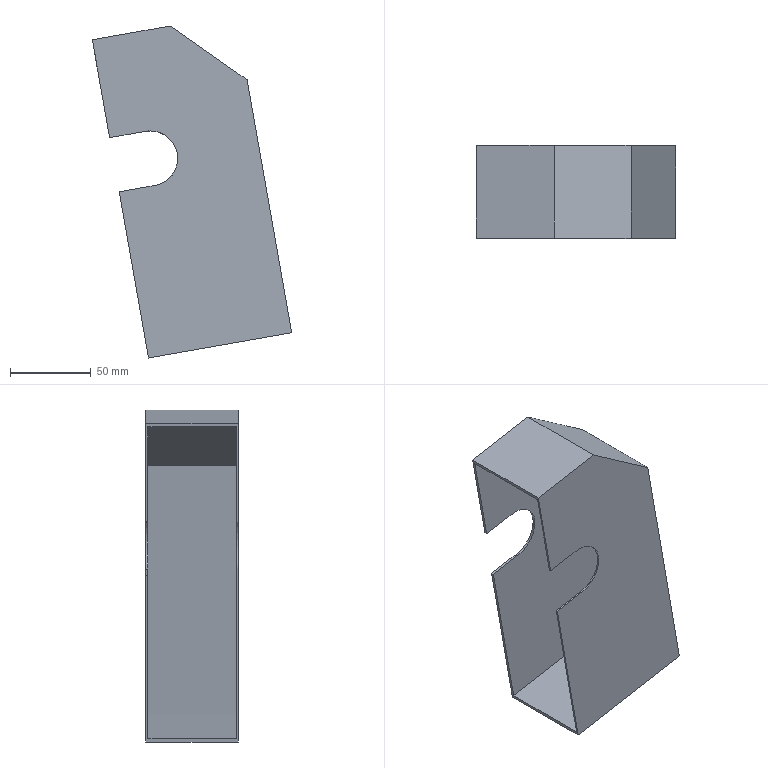Part | SolidWorks | features ICE 3, BaseBody 1, Cut 1 | 1 solid | 21 faces | box 123.362 x 57.5 x 205.47 mm | volume 78596 mm3 | plane 18 | cylinder 3 | commonest cylinder face diameters 34.017 x3
STEP:
#1=CARTESIAN_POINT('',(1.171,250.,328.559));
#2=VERTEX_POINT('',#1);
#3=CARTESIAN_POINT('',(4.125,250.,294.8));
#4=VERTEX_POINT('',#3);
#5=CARTESIAN_POINT('',(1.171,250.,311.55));
#6=DIRECTION('',(0.,1.,0.));
#7=DIRECTION('',(0.,0.,-1.));
#8=AXIS2_PLACEMENT_3D('',#5,#6,#7);
#9=CIRCLE('',#8,17.008);
#10=EDGE_CURVE('',#2,#4,#9,.T.);
#11=ORIENTED_EDGE('',*,*,#10,.F.);
#12=CARTESIAN_POINT('',(1.171,251.,328.559));
#13=VERTEX_POINT('',#12);
#14=CARTESIAN_POINT('',(1.171,191.5,328.559));
#15=DIRECTION('',(0.,1.,0.));
#16=VECTOR('',#15,1000.);
#17=LINE('',#14,#16);
#18=EDGE_CURVE('',#2,#13,#17,.T.);
#19=ORIENTED_EDGE('',*,*,#18,.T.);
#20=CARTESIAN_POINT('',(4.125,251.,294.8));
#21=VERTEX_POINT('',#20);
#22=CARTESIAN_POINT('',(1.171,251.,311.55));
#23=DIRECTION('',(0.,1.,0.));
#24=DIRECTION('',(0.,0.,-1.));
#25=AXIS2_PLACEMENT_3D('',#22,#23,#24);
#26=CIRCLE('',#25,17.008);
#27=EDGE_CURVE('',#13,#21,#26,.T.);
#28=ORIENTED_EDGE('',*,*,#27,.T.);
#29=CARTESIAN_POINT('',(4.125,191.5,294.8));
#30=DIRECTION('',(0.,1.,0.));
#31=VECTOR('',#30,1000.);
#32=LINE('',#29,#31);
#33=EDGE_CURVE('',#4,#21,#32,.T.);
#34=ORIENTED_EDGE('',*,*,#33,.F.);
#35=EDGE_LOOP('',(#11,#19,#28,#34));
#36=FACE_OUTER_BOUND('',#35,.T.);
#37=CARTESIAN_POINT('',(1.171,191.5,311.55));
#38=DIRECTION('',(0.,1.,0.));
#39=DIRECTION('',(0.,0.,1.));
#40=AXIS2_PLACEMENT_3D('',#37,#38,#39);
#41=CYLINDRICAL_SURFACE('',#40,17.008);
#42=ADVANCED_FACE('',(#36),#41,.F.);
#43=CARTESIAN_POINT('',(-18.14,251.,290.874));
#44=VERTEX_POINT('',#43);
#45=CARTESIAN_POINT('',(-18.14,250.,290.874));
#46=VERTEX_POINT('',#45);
#47=CARTESIAN_POINT('',(-18.14,0.,290.874));
#48=DIRECTION('',(0.,-1.,0.));
#49=VECTOR('',#48,1000.);
#50=LINE('',#47,#49);
#51=EDGE_CURVE('',#44,#46,#50,.T.);
#52=ORIENTED_EDGE('',*,*,#51,.F.);
#53=CARTESIAN_POINT('',(-0.3473,251.,189.97));
#54=VERTEX_POINT('',#53);
#55=CARTESIAN_POINT('',(-34.73,251.,384.962));
#56=DIRECTION('',(0.1736,0.,-0.9848));
#57=VECTOR('',#56,1000.);
#58=LINE('',#55,#57);
#59=EDGE_CURVE('',#44,#54,#58,.T.);
#60=ORIENTED_EDGE('',*,*,#59,.T.);
#61=CARTESIAN_POINT('',(-0.3473,306.,189.97));
#62=VERTEX_POINT('',#61);
#63=CARTESIAN_POINT('',(-0.3473,208.,189.97));
#64=DIRECTION('',(0.,1.,0.));
#65=VECTOR('',#64,1000.);
#66=LINE('',#63,#65);
#67=EDGE_CURVE('',#54,#62,#66,.T.);
#68=ORIENTED_EDGE('',*,*,#67,.T.);
#69=CARTESIAN_POINT('',(-18.14,306.,290.874));
#70=VERTEX_POINT('',#69);
#71=CARTESIAN_POINT('',(0.,306.,188.));
#72=DIRECTION('',(-0.1736,0.,0.9848));
#73=VECTOR('',#72,1000.);
#74=LINE('',#71,#73);
#75=EDGE_CURVE('',#62,#70,#74,.T.);
#76=ORIENTED_EDGE('',*,*,#75,.T.);
#77=CARTESIAN_POINT('',(-18.14,307.5,290.874));
#78=VERTEX_POINT('',#77);
#79=CARTESIAN_POINT('',(-18.14,0.,290.874));
#80=DIRECTION('',(0.,1.,0.));
#81=VECTOR('',#80,1000.);
#82=LINE('',#79,#81);
#83=EDGE_CURVE('',#70,#78,#82,.T.);
#84=ORIENTED_EDGE('',*,*,#83,.T.);
#85=CARTESIAN_POINT('',(0.,307.5,188.));
#86=VERTEX_POINT('',#85);
#87=CARTESIAN_POINT('',(0.,307.5,188.));
#88=DIRECTION('',(-0.1736,0.,0.9848));
#89=VECTOR('',#88,1000.);
#90=LINE('',#87,#89);
#91=EDGE_CURVE('',#86,#78,#90,.T.);
#92=ORIENTED_EDGE('',*,*,#91,.F.);
#93=CARTESIAN_POINT('',(0.,250.,188.));
#94=VERTEX_POINT('',#93);
#95=CARTESIAN_POINT('',(0.,208.,188.));
#96=DIRECTION('',(0.,1.,0.));
#97=VECTOR('',#96,1000.);
#98=LINE('',#95,#97);
#99=EDGE_CURVE('',#94,#86,#98,.T.);
#100=ORIENTED_EDGE('',*,*,#99,.F.);
#101=CARTESIAN_POINT('',(-34.73,250.,384.962));
#102=DIRECTION('',(0.1736,0.,-0.9848));
#103=VECTOR('',#102,1000.);
#104=LINE('',#101,#103);
#105=EDGE_CURVE('',#46,#94,#104,.T.);
#106=ORIENTED_EDGE('',*,*,#105,.F.);
#107=EDGE_LOOP('',(#52,#60,#68,#76,#84,#92,#100,#106));
#108=FACE_OUTER_BOUND('',#107,.T.);
#109=CARTESIAN_POINT('',(0.,0.,188.));
#110=DIRECTION('',(0.9848,0.,0.1736));
#111=DIRECTION('',(-0.1736,0.,0.9848));
#112=AXIS2_PLACEMENT_3D('',#109,#110,#111);
#113=PLANE('',#112);
#114=ADVANCED_FACE('',(#108),#113,.F.);
#115=CARTESIAN_POINT('',(-24.046,250.,324.374));
#116=VERTEX_POINT('',#115);
#117=CARTESIAN_POINT('',(-24.046,251.,324.374));
#118=VERTEX_POINT('',#117);
#119=CARTESIAN_POINT('',(-24.046,0.,324.374));
#120=DIRECTION('',(0.,1.,0.));
#121=VECTOR('',#120,1000.);
#122=LINE('',#119,#121);
#123=EDGE_CURVE('',#116,#118,#122,.T.);
#124=ORIENTED_EDGE('',*,*,#123,.F.);
#125=CARTESIAN_POINT('',(-34.73,250.,384.962));
#126=VERTEX_POINT('',#125);
#127=CARTESIAN_POINT('',(-34.73,250.,384.962));
#128=DIRECTION('',(0.1736,0.,-0.9848));
#129=VECTOR('',#128,1000.);
#130=LINE('',#127,#129);
#131=EDGE_CURVE('',#126,#116,#130,.T.);
#132=ORIENTED_EDGE('',*,*,#131,.F.);
#133=CARTESIAN_POINT('',(-34.73,307.5,384.962));
#134=VERTEX_POINT('',#133);
#135=CARTESIAN_POINT('',(-34.73,298.,384.962));
#136=DIRECTION('',(0.,-1.,0.));
#137=VECTOR('',#136,1000.);
#138=LINE('',#135,#137);
#139=EDGE_CURVE('',#134,#126,#138,.T.);
#140=ORIENTED_EDGE('',*,*,#139,.F.);
#141=CARTESIAN_POINT('',(-24.046,307.5,324.374));
#142=VERTEX_POINT('',#141);
#143=CARTESIAN_POINT('',(-24.046,307.5,324.374));
#144=DIRECTION('',(-0.1736,0.,0.9848));
#145=VECTOR('',#144,1000.);
#146=LINE('',#143,#145);
#147=EDGE_CURVE('',#142,#134,#146,.T.);
#148=ORIENTED_EDGE('',*,*,#147,.F.);
#149=CARTESIAN_POINT('',(-24.046,306.,324.374));
#150=VERTEX_POINT('',#149);
#151=CARTESIAN_POINT('',(-24.046,0.,324.374));
#152=DIRECTION('',(0.,-1.,0.));
#153=VECTOR('',#152,1000.);
#154=LINE('',#151,#153);
#155=EDGE_CURVE('',#142,#150,#154,.T.);
#156=ORIENTED_EDGE('',*,*,#155,.T.);
#157=CARTESIAN_POINT('',(-34.382,306.,382.992));
#158=VERTEX_POINT('',#157);
#159=CARTESIAN_POINT('',(0.,306.,188.));
#160=DIRECTION('',(-0.1736,0.,0.9848));
#161=VECTOR('',#160,1000.);
#162=LINE('',#159,#161);
#163=EDGE_CURVE('',#150,#158,#162,.T.);
#164=ORIENTED_EDGE('',*,*,#163,.T.);
#165=CARTESIAN_POINT('',(-34.382,251.,382.992));
#166=VERTEX_POINT('',#165);
#167=CARTESIAN_POINT('',(-34.382,298.,382.992));
#168=DIRECTION('',(0.,-1.,0.));
#169=VECTOR('',#168,1000.);
#170=LINE('',#167,#169);
#171=EDGE_CURVE('',#158,#166,#170,.T.);
#172=ORIENTED_EDGE('',*,*,#171,.T.);
#173=CARTESIAN_POINT('',(-34.73,251.,384.962));
#174=DIRECTION('',(0.1736,0.,-0.9848));
#175=VECTOR('',#174,1000.);
#176=LINE('',#173,#175);
#177=EDGE_CURVE('',#166,#118,#176,.T.);
#178=ORIENTED_EDGE('',*,*,#177,.T.);
#179=EDGE_LOOP('',(#124,#132,#140,#148,#156,#164,#172,#178));
#180=FACE_OUTER_BOUND('',#179,.T.);
#181=CARTESIAN_POINT('',(0.,0.,188.));
#182=DIRECTION('',(0.9848,0.,0.1736));
#183=DIRECTION('',(-0.1736,0.,0.9848));
#184=AXIS2_PLACEMENT_3D('',#181,#182,#183);
#185=PLANE('',#184);
#186=ADVANCED_FACE('',(#180),#185,.F.);
#187=CARTESIAN_POINT('',(-50.289,251.,285.205));
#188=DIRECTION('',(-0.9848,0.,-0.1736));
#189=VECTOR('',#188,1000.);
#190=LINE('',#187,#189);
#191=EDGE_CURVE('',#21,#44,#190,.T.);
#192=ORIENTED_EDGE('',*,*,#191,.F.);
#193=ORIENTED_EDGE('',*,*,#27,.F.);
#194=CARTESIAN_POINT('',(-1.782,251.,328.3));
#195=VERTEX_POINT('',#194);
#196=CARTESIAN_POINT('',(1.171,251.,311.55));
#197=DIRECTION('',(0.,1.,0.));
#198=DIRECTION('',(0.,0.,-1.));
#199=AXIS2_PLACEMENT_3D('',#196,#197,#198);
#200=CIRCLE('',#199,17.008);
#201=EDGE_CURVE('',#195,#13,#200,.T.);
#202=ORIENTED_EDGE('',*,*,#201,.F.);
#203=CARTESIAN_POINT('',(-56.196,251.,318.706));
#204=DIRECTION('',(0.9848,0.,0.1736));
#205=VECTOR('',#204,1000.);
#206=LINE('',#203,#205);
#207=EDGE_CURVE('',#118,#195,#206,.T.);
#208=ORIENTED_EDGE('',*,*,#207,.F.);
#209=ORIENTED_EDGE('',*,*,#177,.F.);
#210=CARTESIAN_POINT('',(13.057,251.,391.357));
#211=VERTEX_POINT('',#210);
#212=CARTESIAN_POINT('',(54.25,251.,398.62));
#213=DIRECTION('',(-0.9848,0.,-0.1736));
#214=VECTOR('',#213,1000.);
#215=LINE('',#212,#214);
#216=EDGE_CURVE('',#211,#166,#215,.T.);
#217=ORIENTED_EDGE('',*,*,#216,.F.);
#218=CARTESIAN_POINT('',(59.197,251.,359.05));
#219=VERTEX_POINT('',#218);
#220=CARTESIAN_POINT('',(59.875,251.,358.574));
#221=DIRECTION('',(0.8192,0.,-0.5736));
#222=VECTOR('',#221,1000.);
#223=LINE('',#220,#222);
#224=EDGE_CURVE('',#211,#219,#223,.T.);
#225=ORIENTED_EDGE('',*,*,#224,.T.);
#226=CARTESIAN_POINT('',(86.316,251.,205.251));
#227=VERTEX_POINT('',#226);
#228=CARTESIAN_POINT('',(86.663,251.,203.281));
#229=DIRECTION('',(0.1736,0.,-0.9848));
#230=VECTOR('',#229,1000.);
#231=LINE('',#228,#230);
#232=EDGE_CURVE('',#219,#227,#231,.T.);
#233=ORIENTED_EDGE('',*,*,#232,.T.);
#234=CARTESIAN_POINT('',(88.285,251.,205.598));
#235=DIRECTION('',(0.9848,0.,0.1736));
#236=VECTOR('',#235,1000.);
#237=LINE('',#234,#236);
#238=EDGE_CURVE('',#54,#227,#237,.T.);
#239=ORIENTED_EDGE('',*,*,#238,.F.);
#240=ORIENTED_EDGE('',*,*,#59,.F.);
#241=EDGE_LOOP('',(#192,#193,#202,#208,#209,#217,#225,#233,#239,#240));
#242=FACE_OUTER_BOUND('',#241,.T.);
#243=CARTESIAN_POINT('',(0.,251.,0.));
#244=DIRECTION('',(0.,-1.,0.));
#245=DIRECTION('',(0.,0.,-1.));
#246=AXIS2_PLACEMENT_3D('',#243,#244,#245);
#247=PLANE('',#246);
#248=ADVANCED_FACE('',(#242),#247,.F.);
#249=CARTESIAN_POINT('',(-1.782,250.,328.3));
#250=VERTEX_POINT('',#249);
#251=CARTESIAN_POINT('',(1.171,250.,311.55));
#252=DIRECTION('',(0.,1.,0.));
#253=DIRECTION('',(0.,0.,-1.));
#254=AXIS2_PLACEMENT_3D('',#251,#252,#253);
#255=CIRCLE('',#254,17.008);
#256=EDGE_CURVE('',#250,#2,#255,.T.);
#257=ORIENTED_EDGE('',*,*,#256,.T.);
#258=ORIENTED_EDGE('',*,*,#10,.T.);
#259=CARTESIAN_POINT('',(-50.289,250.,285.205));
#260=DIRECTION('',(-0.9848,0.,-0.1736));
#261=VECTOR('',#260,1000.);
#262=LINE('',#259,#261);
#263=EDGE_CURVE('',#4,#46,#262,.T.);
#264=ORIENTED_EDGE('',*,*,#263,.T.);
#265=ORIENTED_EDGE('',*,*,#105,.T.);
#266=CARTESIAN_POINT('',(88.633,250.,203.628));
#267=VERTEX_POINT('',#266);
#268=CARTESIAN_POINT('',(0.,250.,188.));
#269=DIRECTION('',(0.9848,0.,0.1736));
#270=VECTOR('',#269,1000.);
#271=LINE('',#268,#270);
#272=EDGE_CURVE('',#94,#267,#271,.T.);
#273=ORIENTED_EDGE('',*,*,#272,.T.);
#274=CARTESIAN_POINT('',(61.023,250.,360.213));
#275=VERTEX_POINT('',#274);
#276=CARTESIAN_POINT('',(88.633,250.,203.628));
#277=DIRECTION('',(-0.1736,0.,0.9848));
#278=VECTOR('',#277,1000.);
#279=LINE('',#276,#278);
#280=EDGE_CURVE('',#267,#275,#279,.T.);
#281=ORIENTED_EDGE('',*,*,#280,.T.);
#282=CARTESIAN_POINT('',(13.526,250.,393.47));
#283=VERTEX_POINT('',#282);
#284=CARTESIAN_POINT('',(61.023,250.,360.213));
#285=DIRECTION('',(-0.8192,0.,0.5736));
#286=VECTOR('',#285,1000.);
#287=LINE('',#284,#286);
#288=EDGE_CURVE('',#275,#283,#287,.T.);
#289=ORIENTED_EDGE('',*,*,#288,.T.);
#290=CARTESIAN_POINT('',(13.526,250.,393.47));
#291=DIRECTION('',(-0.9848,0.,-0.1736));
#292=VECTOR('',#291,1000.);
#293=LINE('',#290,#292);
#294=EDGE_CURVE('',#283,#126,#293,.T.);
#295=ORIENTED_EDGE('',*,*,#294,.T.);
#296=ORIENTED_EDGE('',*,*,#131,.T.);
#297=CARTESIAN_POINT('',(-56.196,250.,318.706));
#298=DIRECTION('',(0.9848,0.,0.1736));
#299=VECTOR('',#298,1000.);
#300=LINE('',#297,#299);
#301=EDGE_CURVE('',#116,#250,#300,.T.);
#302=ORIENTED_EDGE('',*,*,#301,.T.);
#303=EDGE_LOOP('',(#257,#258,#264,#265,#273,#281,#289,#295,#296,#302));
#304=FACE_OUTER_BOUND('',#303,.T.);
#305=CARTESIAN_POINT('',(0.,250.,0.));
#306=DIRECTION('',(0.,-1.,0.));
#307=DIRECTION('',(0.,0.,-1.));
#308=AXIS2_PLACEMENT_3D('',#305,#306,#307);
#309=PLANE('',#308);
#310=ADVANCED_FACE('',(#304),#309,.T.);
#311=CARTESIAN_POINT('',(13.526,307.5,393.47));
#312=VERTEX_POINT('',#311);
#313=CARTESIAN_POINT('',(-34.73,307.5,384.962));
#314=DIRECTION('',(0.9848,0.,0.1736));
#315=VECTOR('',#314,1000.);
#316=LINE('',#313,#315);
#317=EDGE_CURVE('',#134,#312,#316,.T.);
#318=ORIENTED_EDGE('',*,*,#317,.F.);
#319=ORIENTED_EDGE('',*,*,#139,.T.);
#320=ORIENTED_EDGE('',*,*,#294,.F.);
#321=CARTESIAN_POINT('',(13.526,298.,393.47));
#322=DIRECTION('',(0.,1.,0.));
#323=VECTOR('',#322,1000.);
#324=LINE('',#321,#323);
#325=EDGE_CURVE('',#283,#312,#324,.T.);
#326=ORIENTED_EDGE('',*,*,#325,.T.);
#327=EDGE_LOOP('',(#318,#319,#320,#326));
#328=FACE_OUTER_BOUND('',#327,.T.);
#329=CARTESIAN_POINT('',(53.903,298.,400.59));
#330=DIRECTION('',(0.1736,0.,-0.9848));
#331=DIRECTION('',(0.,-1.,0.));
#332=AXIS2_PLACEMENT_3D('',#329,#330,#331);
#333=PLANE('',#332);
#334=ADVANCED_FACE('',(#328),#333,.F.);
#335=CARTESIAN_POINT('',(88.633,307.5,203.628));
#336=VERTEX_POINT('',#335);
#337=CARTESIAN_POINT('',(88.633,307.5,203.628));
#338=DIRECTION('',(-0.9848,0.,-0.1736));
#339=VECTOR('',#338,1000.);
#340=LINE('',#337,#339);
#341=EDGE_CURVE('',#336,#86,#340,.T.);
#342=ORIENTED_EDGE('',*,*,#341,.F.);
#343=CARTESIAN_POINT('',(88.633,208.,203.628));
#344=DIRECTION('',(0.,1.,0.));
#345=VECTOR('',#344,1000.);
#346=LINE('',#343,#345);
#347=EDGE_CURVE('',#267,#336,#346,.T.);
#348=ORIENTED_EDGE('',*,*,#347,.F.);
#349=ORIENTED_EDGE('',*,*,#272,.F.);
#350=ORIENTED_EDGE('',*,*,#99,.T.);
#351=EDGE_LOOP('',(#342,#348,#349,#350));
#352=FACE_OUTER_BOUND('',#351,.T.);
#353=CARTESIAN_POINT('',(88.633,208.,203.628));
#354=DIRECTION('',(-0.1736,0.,0.9848));
#355=DIRECTION('',(0.,1.,0.));
#356=AXIS2_PLACEMENT_3D('',#353,#354,#355);
#357=PLANE('',#356);
#358=ADVANCED_FACE('',(#352),#357,.F.);
#359=ORIENTED_EDGE('',*,*,#347,.T.);
#360=CARTESIAN_POINT('',(61.023,307.5,360.213));
#361=VERTEX_POINT('',#360);
#362=CARTESIAN_POINT('',(61.023,307.5,360.213));
#363=DIRECTION('',(0.1736,0.,-0.9848));
#364=VECTOR('',#363,1000.);
#365=LINE('',#362,#364);
#366=EDGE_CURVE('',#361,#336,#365,.T.);
#367=ORIENTED_EDGE('',*,*,#366,.F.);
#368=CARTESIAN_POINT('',(61.023,208.,360.213));
#369=DIRECTION('',(0.,-1.,0.));
#370=VECTOR('',#369,1000.);
#371=LINE('',#368,#370);
#372=EDGE_CURVE('',#361,#275,#371,.T.);
#373=ORIENTED_EDGE('',*,*,#372,.T.);
#374=ORIENTED_EDGE('',*,*,#280,.F.);
#375=EDGE_LOOP('',(#359,#367,#373,#374));
#376=FACE_OUTER_BOUND('',#375,.T.);
#377=CARTESIAN_POINT('',(88.633,0.,203.628));
#378=DIRECTION('',(0.9848,0.,0.1736));
#379=DIRECTION('',(-0.1736,0.,0.9848));
#380=AXIS2_PLACEMENT_3D('',#377,#378,#379);
#381=PLANE('',#380);
#382=ADVANCED_FACE('',(#376),#381,.T.);
#383=ORIENTED_EDGE('',*,*,#372,.F.);
#384=CARTESIAN_POINT('',(13.526,307.5,393.47));
#385=DIRECTION('',(0.8192,0.,-0.5736));
#386=VECTOR('',#385,1000.);
#387=LINE('',#384,#386);
#388=EDGE_CURVE('',#312,#361,#387,.T.);
#389=ORIENTED_EDGE('',*,*,#388,.F.);
#390=ORIENTED_EDGE('',*,*,#325,.F.);
#391=ORIENTED_EDGE('',*,*,#288,.F.);
#392=EDGE_LOOP('',(#383,#389,#390,#391));
#393=FACE_OUTER_BOUND('',#392,.T.);
#394=CARTESIAN_POINT('',(61.023,0.,360.213));
#395=DIRECTION('',(0.5736,0.,0.8192));
#396=DIRECTION('',(0.,-1.,0.));
#397=AXIS2_PLACEMENT_3D('',#394,#395,#396);
#398=PLANE('',#397);
#399=ADVANCED_FACE('',(#393),#398,.T.);
#400=CARTESIAN_POINT('',(4.125,307.5,294.8));
#401=VERTEX_POINT('',#400);
#402=CARTESIAN_POINT('',(-1.782,307.5,328.3));
#403=VERTEX_POINT('',#402);
#404=CARTESIAN_POINT('',(1.171,307.5,311.55));
#405=DIRECTION('',(0.,-1.,0.));
#406=DIRECTION('',(0.,0.,1.));
#407=AXIS2_PLACEMENT_3D('',#404,#405,#406);
#408=CIRCLE('',#407,17.008);
#409=EDGE_CURVE('',#401,#403,#408,.T.);
#410=ORIENTED_EDGE('',*,*,#409,.F.);
#411=CARTESIAN_POINT('',(4.125,306.,294.8));
#412=VERTEX_POINT('',#411);
#413=CARTESIAN_POINT('',(4.125,283.,294.8));
#414=DIRECTION('',(0.,1.,0.));
#415=VECTOR('',#414,1000.);
#416=LINE('',#413,#415);
#417=EDGE_CURVE('',#412,#401,#416,.T.);
#418=ORIENTED_EDGE('',*,*,#417,.F.);
#419=CARTESIAN_POINT('',(-1.782,306.,328.3));
#420=VERTEX_POINT('',#419);
#421=CARTESIAN_POINT('',(1.171,306.,311.55));
#422=DIRECTION('',(0.,-1.,0.));
#423=DIRECTION('',(0.1736,0.,-0.9848));
#424=AXIS2_PLACEMENT_3D('',#421,#422,#423);
#425=CIRCLE('',#424,17.008);
#426=EDGE_CURVE('',#412,#420,#425,.T.);
#427=ORIENTED_EDGE('',*,*,#426,.T.);
#428=CARTESIAN_POINT('',(-1.782,283.,328.3));
#429=DIRECTION('',(0.,1.,0.));
#430=VECTOR('',#429,1000.);
#431=LINE('',#428,#430);
#432=EDGE_CURVE('',#420,#403,#431,.T.);
#433=ORIENTED_EDGE('',*,*,#432,.T.);
#434=EDGE_LOOP('',(#410,#418,#427,#433));
#435=FACE_OUTER_BOUND('',#434,.T.);
#436=CARTESIAN_POINT('',(1.171,238.,311.55));
#437=DIRECTION('',(0.,1.,0.));
#438=DIRECTION('',(-0.9848,0.,-0.1736));
#439=AXIS2_PLACEMENT_3D('',#436,#437,#438);
#440=CYLINDRICAL_SURFACE('',#439,17.008);
#441=ADVANCED_FACE('',(#435),#440,.F.);
#442=CARTESIAN_POINT('',(-18.14,307.5,290.874));
#443=DIRECTION('',(0.9848,0.,0.1736));
#444=VECTOR('',#443,1000.);
#445=LINE('',#442,#444);
#446=EDGE_CURVE('',#78,#401,#445,.T.);
#447=ORIENTED_EDGE('',*,*,#446,.F.);
#448=ORIENTED_EDGE('',*,*,#83,.F.);
#449=CARTESIAN_POINT('',(70.493,306.,306.503));
#450=DIRECTION('',(0.9848,0.,0.1736));
#451=VECTOR('',#450,1000.);
#452=LINE('',#449,#451);
#453=EDGE_CURVE('',#70,#412,#452,.T.);
#454=ORIENTED_EDGE('',*,*,#453,.T.);
#455=ORIENTED_EDGE('',*,*,#417,.T.);
#456=EDGE_LOOP('',(#447,#448,#454,#455));
#457=FACE_OUTER_BOUND('',#456,.T.);
#458=CARTESIAN_POINT('',(4.125,283.,294.8));
#459=DIRECTION('',(0.1736,0.,-0.9848));
#460=DIRECTION('',(0.9848,0.,0.1736));
#461=AXIS2_PLACEMENT_3D('',#458,#459,#460);
#462=PLANE('',#461);
#463=ADVANCED_FACE('',(#457),#462,.F.);
#464=CARTESIAN_POINT('',(-1.782,307.5,328.3));
#465=DIRECTION('',(-0.9848,0.,-0.1736));
#466=VECTOR('',#465,1000.);
#467=LINE('',#464,#466);
#468=EDGE_CURVE('',#403,#142,#467,.T.);
#469=ORIENTED_EDGE('',*,*,#468,.F.);
#470=ORIENTED_EDGE('',*,*,#432,.F.);
#471=CARTESIAN_POINT('',(64.586,306.,340.003));
#472=DIRECTION('',(-0.9848,0.,-0.1736));
#473=VECTOR('',#472,1000.);
#474=LINE('',#471,#473);
#475=EDGE_CURVE('',#420,#150,#474,.T.);
#476=ORIENTED_EDGE('',*,*,#475,.T.);
#477=ORIENTED_EDGE('',*,*,#155,.F.);
#478=EDGE_LOOP('',(#469,#470,#476,#477));
#479=FACE_OUTER_BOUND('',#478,.T.);
#480=CARTESIAN_POINT('',(-49.541,283.,319.879));
#481=DIRECTION('',(-0.1736,0.,0.9848));
#482=DIRECTION('',(-0.9848,0.,-0.1736));
#483=AXIS2_PLACEMENT_3D('',#480,#481,#482);
#484=PLANE('',#483);
#485=ADVANCED_FACE('',(#479),#484,.F.);
#486=CARTESIAN_POINT('',(13.057,306.,391.357));
#487=VERTEX_POINT('',#486);
#488=CARTESIAN_POINT('',(13.057,0.,391.357));
#489=DIRECTION('',(0.,1.,0.));
#490=VECTOR('',#489,1000.);
#491=LINE('',#488,#490);
#492=EDGE_CURVE('',#211,#487,#491,.T.);
#493=ORIENTED_EDGE('',*,*,#492,.F.);
#494=ORIENTED_EDGE('',*,*,#216,.T.);
#495=ORIENTED_EDGE('',*,*,#171,.F.);
#496=CARTESIAN_POINT('',(54.25,306.,398.62));
#497=DIRECTION('',(-0.9848,0.,-0.1736));
#498=VECTOR('',#497,1000.);
#499=LINE('',#496,#498);
#500=EDGE_CURVE('',#487,#158,#499,.T.);
#501=ORIENTED_EDGE('',*,*,#500,.F.);
#502=EDGE_LOOP('',(#493,#494,#495,#501));
#503=FACE_OUTER_BOUND('',#502,.T.);
#504=CARTESIAN_POINT('',(54.25,298.,398.62));
#505=DIRECTION('',(0.1736,0.,-0.9848));
#506=DIRECTION('',(0.,-1.,0.));
#507=AXIS2_PLACEMENT_3D('',#504,#505,#506);
#508=PLANE('',#507);
#509=ADVANCED_FACE('',(#503),#508,.T.);
#510=ORIENTED_EDGE('',*,*,#67,.F.);
#511=ORIENTED_EDGE('',*,*,#238,.T.);
#512=CARTESIAN_POINT('',(86.316,306.,205.251));
#513=VERTEX_POINT('',#512);
#514=CARTESIAN_POINT('',(86.316,208.,205.251));
#515=DIRECTION('',(0.,1.,0.));
#516=VECTOR('',#515,1000.);
#517=LINE('',#514,#516);
#518=EDGE_CURVE('',#227,#513,#517,.T.);
#519=ORIENTED_EDGE('',*,*,#518,.T.);
#520=CARTESIAN_POINT('',(88.285,306.,205.598));
#521=DIRECTION('',(-0.9848,0.,-0.1736));
#522=VECTOR('',#521,1000.);
#523=LINE('',#520,#522);
#524=EDGE_CURVE('',#513,#62,#523,.T.);
#525=ORIENTED_EDGE('',*,*,#524,.T.);
#526=EDGE_LOOP('',(#510,#511,#519,#525));
#527=FACE_OUTER_BOUND('',#526,.T.);
#528=CARTESIAN_POINT('',(88.285,208.,205.598));
#529=DIRECTION('',(-0.1736,0.,0.9848));
#530=DIRECTION('',(0.,1.,0.));
#531=AXIS2_PLACEMENT_3D('',#528,#529,#530);
#532=PLANE('',#531);
#533=ADVANCED_FACE('',(#527),#532,.T.);
#534=ORIENTED_EDGE('',*,*,#232,.F.);
#535=CARTESIAN_POINT('',(59.197,306.,359.05));
#536=VERTEX_POINT('',#535);
#537=CARTESIAN_POINT('',(59.197,0.,359.05));
#538=DIRECTION('',(0.,-1.,0.));
#539=VECTOR('',#538,1000.);
#540=LINE('',#537,#539);
#541=EDGE_CURVE('',#536,#219,#540,.T.);
#542=ORIENTED_EDGE('',*,*,#541,.F.);
#543=CARTESIAN_POINT('',(86.663,306.,203.281));
#544=DIRECTION('',(-0.1736,0.,0.9848));
#545=VECTOR('',#544,1000.);
#546=LINE('',#543,#545);
#547=EDGE_CURVE('',#513,#536,#546,.T.);
#548=ORIENTED_EDGE('',*,*,#547,.F.);
#549=ORIENTED_EDGE('',*,*,#518,.F.);
#550=EDGE_LOOP('',(#534,#542,#548,#549));
#551=FACE_OUTER_BOUND('',#550,.T.);
#552=CARTESIAN_POINT('',(86.663,0.,203.281));
#553=DIRECTION('',(0.9848,0.,0.1736));
#554=DIRECTION('',(-0.1736,0.,0.9848));
#555=AXIS2_PLACEMENT_3D('',#552,#553,#554);
#556=PLANE('',#555);
#557=ADVANCED_FACE('',(#551),#556,.F.);
#558=ORIENTED_EDGE('',*,*,#224,.F.);
#559=ORIENTED_EDGE('',*,*,#492,.T.);
#560=CARTESIAN_POINT('',(59.875,306.,358.574));
#561=DIRECTION('',(0.8192,0.,-0.5736));
#562=VECTOR('',#561,1000.);
#563=LINE('',#560,#562);
#564=EDGE_CURVE('',#487,#536,#563,.T.);
#565=ORIENTED_EDGE('',*,*,#564,.T.);
#566=ORIENTED_EDGE('',*,*,#541,.T.);
#567=EDGE_LOOP('',(#558,#559,#565,#566));
#568=FACE_OUTER_BOUND('',#567,.T.);
#569=CARTESIAN_POINT('',(59.875,0.,358.574));
#570=DIRECTION('',(0.5736,0.,0.8192));
#571=DIRECTION('',(0.,-1.,0.));
#572=AXIS2_PLACEMENT_3D('',#569,#570,#571);
#573=PLANE('',#572);
#574=ADVANCED_FACE('',(#568),#573,.F.);
#575=ORIENTED_EDGE('',*,*,#475,.F.);
#576=ORIENTED_EDGE('',*,*,#426,.F.);
#577=ORIENTED_EDGE('',*,*,#453,.F.);
#578=ORIENTED_EDGE('',*,*,#75,.F.);
#579=ORIENTED_EDGE('',*,*,#524,.F.);
#580=ORIENTED_EDGE('',*,*,#547,.T.);
#581=ORIENTED_EDGE('',*,*,#564,.F.);
#582=ORIENTED_EDGE('',*,*,#500,.T.);
#583=ORIENTED_EDGE('',*,*,#163,.F.);
#584=EDGE_LOOP('',(#575,#576,#577,#578,#579,#580,#581,#582,#583));
#585=FACE_OUTER_BOUND('',#584,.T.);
#586=CARTESIAN_POINT('',(88.633,306.,203.628));
#587=DIRECTION('',(0.,-1.,0.));
#588=DIRECTION('',(-0.1736,0.,0.9848));
#589=AXIS2_PLACEMENT_3D('',#586,#587,#588);
#590=PLANE('',#589);
#591=ADVANCED_FACE('',(#585),#590,.T.);
#592=ORIENTED_EDGE('',*,*,#409,.T.);
#593=ORIENTED_EDGE('',*,*,#468,.T.);
#594=ORIENTED_EDGE('',*,*,#147,.T.);
#595=ORIENTED_EDGE('',*,*,#317,.T.);
#596=ORIENTED_EDGE('',*,*,#388,.T.);
#597=ORIENTED_EDGE('',*,*,#366,.T.);
#598=ORIENTED_EDGE('',*,*,#341,.T.);
#599=ORIENTED_EDGE('',*,*,#91,.T.);
#600=ORIENTED_EDGE('',*,*,#446,.T.);
#601=EDGE_LOOP('',(#592,#593,#594,#595,#596,#597,#598,#599,#600));
#602=FACE_OUTER_BOUND('',#601,.T.);
#603=CARTESIAN_POINT('',(1.171,307.5,311.55));
#604=DIRECTION('',(0.,1.,0.));
#605=DIRECTION('',(0.,0.,1.));
#606=AXIS2_PLACEMENT_3D('',#603,#604,#605);
#607=PLANE('',#606);
#608=ADVANCED_FACE('',(#602),#607,.T.);
#609=ORIENTED_EDGE('',*,*,#191,.T.);
#610=ORIENTED_EDGE('',*,*,#51,.T.);
#611=ORIENTED_EDGE('',*,*,#263,.F.);
#612=ORIENTED_EDGE('',*,*,#33,.T.);
#613=EDGE_LOOP('',(#609,#610,#611,#612));
#614=FACE_OUTER_BOUND('',#613,.T.);
#615=CARTESIAN_POINT('',(-50.289,191.5,285.205));
#616=DIRECTION('',(-0.1736,0.,0.9848));
#617=DIRECTION('',(0.9848,0.,0.1736));
#618=AXIS2_PLACEMENT_3D('',#615,#616,#617);
#619=PLANE('',#618);
#620=ADVANCED_FACE('',(#614),#619,.T.);
#621=ORIENTED_EDGE('',*,*,#18,.F.);
#622=ORIENTED_EDGE('',*,*,#256,.F.);
#623=CARTESIAN_POINT('',(-1.782,191.5,328.3));
#624=DIRECTION('',(0.,1.,0.));
#625=VECTOR('',#624,1000.);
#626=LINE('',#623,#625);
#627=EDGE_CURVE('',#250,#195,#626,.T.);
#628=ORIENTED_EDGE('',*,*,#627,.T.);
#629=ORIENTED_EDGE('',*,*,#201,.T.);
#630=EDGE_LOOP('',(#621,#622,#628,#629));
#631=FACE_OUTER_BOUND('',#630,.T.);
#632=CARTESIAN_POINT('',(1.171,191.5,311.55));
#633=DIRECTION('',(0.,1.,0.));
#634=DIRECTION('',(0.,0.,1.));
#635=AXIS2_PLACEMENT_3D('',#632,#633,#634);
#636=CYLINDRICAL_SURFACE('',#635,17.008);
#637=ADVANCED_FACE('',(#631),#636,.F.);
#638=ORIENTED_EDGE('',*,*,#207,.T.);
#639=ORIENTED_EDGE('',*,*,#627,.F.);
#640=ORIENTED_EDGE('',*,*,#301,.F.);
#641=ORIENTED_EDGE('',*,*,#123,.T.);
#642=EDGE_LOOP('',(#638,#639,#640,#641));
#643=FACE_OUTER_BOUND('',#642,.T.);
#644=CARTESIAN_POINT('',(-56.196,191.5,318.706));
#645=DIRECTION('',(0.1736,0.,-0.9848));
#646=DIRECTION('',(-0.9848,0.,-0.1736));
#647=AXIS2_PLACEMENT_3D('',#644,#645,#646);
#648=PLANE('',#647);
#649=ADVANCED_FACE('',(#643),#648,.T.);
#650=CLOSED_SHELL('',(#42,#114,#186,#248,#310,#334,#358,#382,#399,#441,#463,#485,#509,#533,#557,#574,#591,#608,#620,#637,#649));
#651=MANIFOLD_SOLID_BREP('',#650);
#652=CARTESIAN_POINT('',(0.,0.,0.));
#653=DIRECTION('',(0.,0.,1.));
#654=DIRECTION('',(1.,0.,0.));
#655=AXIS2_PLACEMENT_3D('',#652,#653,#654);
#656=(LENGTH_UNIT()NAMED_UNIT(*)SI_UNIT(.MILLI.,.METRE.));
#657=UNCERTAINTY_MEASURE_WITH_UNIT(LENGTH_MEASURE(0.00001),#656,'','');
#658=(NAMED_UNIT(*)PLANE_ANGLE_UNIT()SI_UNIT($,.RADIAN.));
#659=(NAMED_UNIT(*)SI_UNIT($,.STERADIAN.)SOLID_ANGLE_UNIT());
#660=(GEOMETRIC_REPRESENTATION_CONTEXT(3)GLOBAL_UNCERTAINTY_ASSIGNED_CONTEXT((#657))GLOBAL_UNIT_ASSIGNED_CONTEXT((#656,#658,#659))REPRESENTATION_CONTEXT('',''));
#661=ADVANCED_BREP_SHAPE_REPRESENTATION('',(#651,#655),#660);